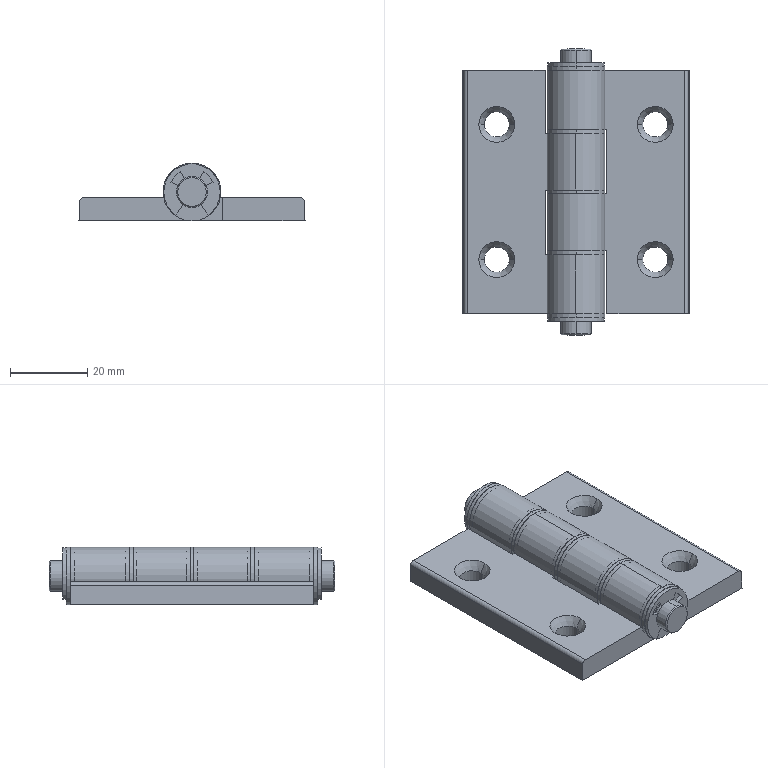Part | STEP file | LE-LHY-40A_LE0314002639 | 18 solids | 252 faces | box 58.5 x 74 x 15 mm | volume 28707 mm3 | cylinder 124 | plane 116 | cone 12 | commonest cylinder face diameters 7.2 x39 8 x24 12 x20 15 x16 14.6 x15 6.5 x8